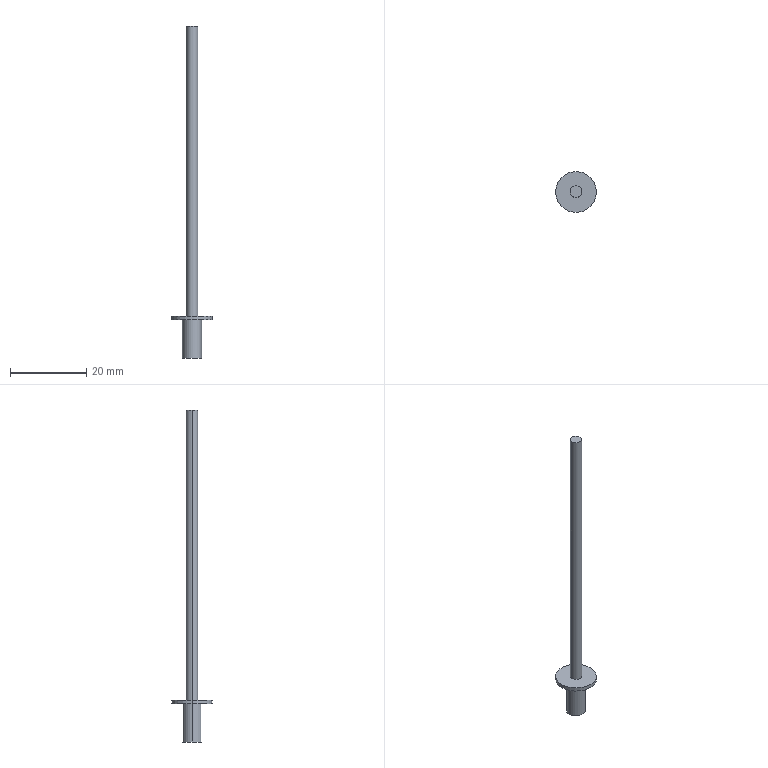Part | Creo | 1 solid | 10 faces | box 10.7 x 10.7 x 87 mm | volume 823.482 mm3 | cylinder 6 | plane 4 | commonest cylinder face diameters 3 x2 5 x2 10.7 x2
STEP:
#1=CARTESIAN_POINT('',(0.,0.,0.));
#2=DIRECTION('',(0.,0.,1.));
#3=DIRECTION('',(1.,0.,0.));
#4=AXIS2_PLACEMENT_3D('',#1,#2,#3);
#5=CARTESIAN_POINT('',(-34.3,80.134,-54.09));
#6=VERTEX_POINT('',#5);
#7=CARTESIAN_POINT('',(-31.3,80.134,-54.09));
#8=VERTEX_POINT('',#7);
#9=CARTESIAN_POINT('',(-32.8,80.134,-54.09));
#10=DIRECTION('',(0.,0.,-1.));
#11=DIRECTION('',(-1.,0.,0.));
#12=AXIS2_PLACEMENT_3D('',#9,#10,#11);
#13=CIRCLE('',#12,1.5);
#14=EDGE_CURVE('',#6,#8,#13,.T.);
#15=ORIENTED_EDGE('',*,*,#14,.T.);
#16=CARTESIAN_POINT('',(-31.3,80.134,21.91));
#17=VERTEX_POINT('',#16);
#18=CARTESIAN_POINT('',(-31.3,80.134,21.91));
#19=DIRECTION('',(0.,0.,-1.));
#20=VECTOR('',#19,76.);
#21=LINE('',#18,#20);
#22=EDGE_CURVE('',#17,#8,#21,.T.);
#23=ORIENTED_EDGE('',*,*,#22,.F.);
#24=CARTESIAN_POINT('',(-34.3,80.134,21.91));
#25=VERTEX_POINT('',#24);
#26=CARTESIAN_POINT('',(-32.8,80.134,21.91));
#27=DIRECTION('',(0.,0.,1.));
#28=DIRECTION('',(1.,0.,0.));
#29=AXIS2_PLACEMENT_3D('',#26,#27,#28);
#30=CIRCLE('',#29,1.5);
#31=EDGE_CURVE('',#17,#25,#30,.T.);
#32=ORIENTED_EDGE('',*,*,#31,.T.);
#33=CARTESIAN_POINT('',(-34.3,80.134,21.91));
#34=DIRECTION('',(0.,0.,-1.));
#35=VECTOR('',#34,76.);
#36=LINE('',#33,#35);
#37=EDGE_CURVE('',#25,#6,#36,.T.);
#38=ORIENTED_EDGE('',*,*,#37,.T.);
#39=EDGE_LOOP('',(#15,#23,#32,#38));
#40=FACE_OUTER_BOUND('',#39,.F.);
#41=CARTESIAN_POINT('',(-32.8,80.134,10.91));
#42=DIRECTION('',(0.,0.,-1.));
#43=DIRECTION('',(-1.,0.,0.));
#44=AXIS2_PLACEMENT_3D('',#41,#42,#43);
#45=CYLINDRICAL_SURFACE('',#44,1.5);
#46=ADVANCED_FACE('',(#40),#45,.T.);
#47=CARTESIAN_POINT('',(-38.15,80.134,-54.09));
#48=VERTEX_POINT('',#47);
#49=CARTESIAN_POINT('',(-27.45,80.134,-54.09));
#50=VERTEX_POINT('',#49);
#51=CARTESIAN_POINT('',(-32.8,80.134,-54.09));
#52=DIRECTION('',(0.,0.,1.));
#53=DIRECTION('',(-1.,0.,0.));
#54=AXIS2_PLACEMENT_3D('',#51,#52,#53);
#55=CIRCLE('',#54,5.35);
#56=EDGE_CURVE('',#48,#50,#55,.T.);
#57=ORIENTED_EDGE('',*,*,#56,.F.);
#58=CARTESIAN_POINT('',(-32.8,80.134,-54.09));
#59=DIRECTION('',(0.,0.,1.));
#60=DIRECTION('',(1.,0.,0.));
#61=AXIS2_PLACEMENT_3D('',#58,#59,#60);
#62=CIRCLE('',#61,5.35);
#63=EDGE_CURVE('',#50,#48,#62,.T.);
#64=ORIENTED_EDGE('',*,*,#63,.F.);
#65=EDGE_LOOP('',(#57,#64));
#66=FACE_OUTER_BOUND('',#65,.F.);
#67=ORIENTED_EDGE('',*,*,#14,.F.);
#68=CARTESIAN_POINT('',(-32.8,80.134,-54.09));
#69=DIRECTION('',(0.,0.,-1.));
#70=DIRECTION('',(1.,0.,0.));
#71=AXIS2_PLACEMENT_3D('',#68,#69,#70);
#72=CIRCLE('',#71,1.5);
#73=EDGE_CURVE('',#8,#6,#72,.T.);
#74=ORIENTED_EDGE('',*,*,#73,.F.);
#75=EDGE_LOOP('',(#67,#74));
#76=FACE_BOUND('',#75,.F.);
#77=CARTESIAN_POINT('',(0.,0.,-54.09));
#78=DIRECTION('',(0.,0.,-1.));
#79=DIRECTION('',(-1.,0.,0.));
#80=AXIS2_PLACEMENT_3D('',#77,#78,#79);
#81=PLANE('',#80);
#82=ADVANCED_FACE('',(#66,#76),#81,.F.);
#83=ORIENTED_EDGE('',*,*,#56,.T.);
#84=CARTESIAN_POINT('',(-27.45,80.134,-55.09));
#85=VERTEX_POINT('',#84);
#86=CARTESIAN_POINT('',(-27.45,80.134,-55.09));
#87=DIRECTION('',(0.,0.,1.));
#88=VECTOR('',#87,1.);
#89=LINE('',#86,#88);
#90=EDGE_CURVE('',#85,#50,#89,.T.);
#91=ORIENTED_EDGE('',*,*,#90,.F.);
#92=CARTESIAN_POINT('',(-38.15,80.134,-55.09));
#93=VERTEX_POINT('',#92);
#94=CARTESIAN_POINT('',(-32.8,80.134,-55.09));
#95=DIRECTION('',(0.,0.,-1.));
#96=DIRECTION('',(1.,0.,0.));
#97=AXIS2_PLACEMENT_3D('',#94,#95,#96);
#98=CIRCLE('',#97,5.35);
#99=EDGE_CURVE('',#85,#93,#98,.T.);
#100=ORIENTED_EDGE('',*,*,#99,.T.);
#101=CARTESIAN_POINT('',(-38.15,80.134,-55.09));
#102=DIRECTION('',(0.,0.,1.));
#103=VECTOR('',#102,1.);
#104=LINE('',#101,#103);
#105=EDGE_CURVE('',#93,#48,#104,.T.);
#106=ORIENTED_EDGE('',*,*,#105,.T.);
#107=EDGE_LOOP('',(#83,#91,#100,#106));
#108=FACE_OUTER_BOUND('',#107,.F.);
#109=CARTESIAN_POINT('',(-32.8,80.134,-104.09));
#110=DIRECTION('',(0.,0.,1.));
#111=DIRECTION('',(1.,0.,0.));
#112=AXIS2_PLACEMENT_3D('',#109,#110,#111);
#113=CYLINDRICAL_SURFACE('',#112,5.35);
#114=ADVANCED_FACE('',(#108),#113,.T.);
#115=ORIENTED_EDGE('',*,*,#63,.T.);
#116=ORIENTED_EDGE('',*,*,#105,.F.);
#117=CARTESIAN_POINT('',(-32.8,80.134,-55.09));
#118=DIRECTION('',(0.,0.,-1.));
#119=DIRECTION('',(-1.,0.,0.));
#120=AXIS2_PLACEMENT_3D('',#117,#118,#119);
#121=CIRCLE('',#120,5.35);
#122=EDGE_CURVE('',#93,#85,#121,.T.);
#123=ORIENTED_EDGE('',*,*,#122,.T.);
#124=ORIENTED_EDGE('',*,*,#90,.T.);
#125=EDGE_LOOP('',(#115,#116,#123,#124));
#126=FACE_OUTER_BOUND('',#125,.F.);
#127=CARTESIAN_POINT('',(-32.8,80.134,-104.09));
#128=DIRECTION('',(0.,0.,1.));
#129=DIRECTION('',(1.,0.,0.));
#130=AXIS2_PLACEMENT_3D('',#127,#128,#129);
#131=CYLINDRICAL_SURFACE('',#130,5.35);
#132=ADVANCED_FACE('',(#126),#131,.T.);
#133=ORIENTED_EDGE('',*,*,#122,.F.);
#134=ORIENTED_EDGE('',*,*,#99,.F.);
#135=EDGE_LOOP('',(#133,#134));
#136=FACE_OUTER_BOUND('',#135,.F.);
#137=CARTESIAN_POINT('',(-35.3,80.134,-55.09));
#138=VERTEX_POINT('',#137);
#139=CARTESIAN_POINT('',(-30.3,80.134,-55.09));
#140=VERTEX_POINT('',#139);
#141=CARTESIAN_POINT('',(-32.8,80.134,-55.09));
#142=DIRECTION('',(0.,0.,1.));
#143=DIRECTION('',(-1.,0.,0.));
#144=AXIS2_PLACEMENT_3D('',#141,#142,#143);
#145=CIRCLE('',#144,2.5);
#146=EDGE_CURVE('',#138,#140,#145,.T.);
#147=ORIENTED_EDGE('',*,*,#146,.F.);
#148=CARTESIAN_POINT('',(-32.8,80.134,-55.09));
#149=DIRECTION('',(0.,0.,1.));
#150=DIRECTION('',(1.,0.,0.));
#151=AXIS2_PLACEMENT_3D('',#148,#149,#150);
#152=CIRCLE('',#151,2.5);
#153=EDGE_CURVE('',#140,#138,#152,.T.);
#154=ORIENTED_EDGE('',*,*,#153,.F.);
#155=EDGE_LOOP('',(#147,#154));
#156=FACE_BOUND('',#155,.F.);
#157=CARTESIAN_POINT('',(0.,0.,-55.09));
#158=DIRECTION('',(0.,0.,-1.));
#159=DIRECTION('',(-1.,0.,0.));
#160=AXIS2_PLACEMENT_3D('',#157,#158,#159);
#161=PLANE('',#160);
#162=ADVANCED_FACE('',(#136,#156),#161,.T.);
#163=CARTESIAN_POINT('',(-30.3,80.134,-65.09));
#164=VERTEX_POINT('',#163);
#165=CARTESIAN_POINT('',(-35.3,80.134,-65.09));
#166=VERTEX_POINT('',#165);
#167=CARTESIAN_POINT('',(-32.8,80.134,-65.09));
#168=DIRECTION('',(0.,0.,-1.));
#169=DIRECTION('',(1.,0.,0.));
#170=AXIS2_PLACEMENT_3D('',#167,#168,#169);
#171=CIRCLE('',#170,2.5);
#172=EDGE_CURVE('',#164,#166,#171,.T.);
#173=ORIENTED_EDGE('',*,*,#172,.T.);
#174=CARTESIAN_POINT('',(-35.3,80.134,-55.09));
#175=DIRECTION('',(0.,0.,-1.));
#176=VECTOR('',#175,10.);
#177=LINE('',#174,#176);
#178=EDGE_CURVE('',#138,#166,#177,.T.);
#179=ORIENTED_EDGE('',*,*,#178,.F.);
#180=ORIENTED_EDGE('',*,*,#146,.T.);
#181=CARTESIAN_POINT('',(-30.3,80.134,-55.09));
#182=DIRECTION('',(0.,0.,-1.));
#183=VECTOR('',#182,10.);
#184=LINE('',#181,#183);
#185=EDGE_CURVE('',#140,#164,#184,.T.);
#186=ORIENTED_EDGE('',*,*,#185,.T.);
#187=EDGE_LOOP('',(#173,#179,#180,#186));
#188=FACE_OUTER_BOUND('',#187,.F.);
#189=CARTESIAN_POINT('',(-32.8,80.134,-55.09));
#190=DIRECTION('',(0.,0.,-1.));
#191=DIRECTION('',(-1.,0.,0.));
#192=AXIS2_PLACEMENT_3D('',#189,#190,#191);
#193=CYLINDRICAL_SURFACE('',#192,2.5);
#194=ADVANCED_FACE('',(#188),#193,.T.);
#195=ORIENTED_EDGE('',*,*,#172,.F.);
#196=CARTESIAN_POINT('',(-32.8,80.134,-65.09));
#197=DIRECTION('',(0.,0.,-1.));
#198=DIRECTION('',(-1.,0.,0.));
#199=AXIS2_PLACEMENT_3D('',#196,#197,#198);
#200=CIRCLE('',#199,2.5);
#201=EDGE_CURVE('',#166,#164,#200,.T.);
#202=ORIENTED_EDGE('',*,*,#201,.F.);
#203=EDGE_LOOP('',(#195,#202));
#204=FACE_OUTER_BOUND('',#203,.F.);
#205=CARTESIAN_POINT('',(-32.8,80.134,-65.09));
#206=DIRECTION('',(0.,0.,1.));
#207=DIRECTION('',(1.,0.,0.));
#208=AXIS2_PLACEMENT_3D('',#205,#206,#207);
#209=PLANE('',#208);
#210=ADVANCED_FACE('',(#204),#209,.F.);
#211=ORIENTED_EDGE('',*,*,#201,.T.);
#212=ORIENTED_EDGE('',*,*,#185,.F.);
#213=ORIENTED_EDGE('',*,*,#153,.T.);
#214=ORIENTED_EDGE('',*,*,#178,.T.);
#215=EDGE_LOOP('',(#211,#212,#213,#214));
#216=FACE_OUTER_BOUND('',#215,.F.);
#217=CARTESIAN_POINT('',(-32.8,80.134,-55.09));
#218=DIRECTION('',(0.,0.,-1.));
#219=DIRECTION('',(-1.,0.,0.));
#220=AXIS2_PLACEMENT_3D('',#217,#218,#219);
#221=CYLINDRICAL_SURFACE('',#220,2.5);
#222=ADVANCED_FACE('',(#216),#221,.T.);
#223=ORIENTED_EDGE('',*,*,#73,.T.);
#224=ORIENTED_EDGE('',*,*,#37,.F.);
#225=CARTESIAN_POINT('',(-32.8,80.134,21.91));
#226=DIRECTION('',(0.,0.,1.));
#227=DIRECTION('',(-1.,0.,0.));
#228=AXIS2_PLACEMENT_3D('',#225,#226,#227);
#229=CIRCLE('',#228,1.5);
#230=EDGE_CURVE('',#25,#17,#229,.T.);
#231=ORIENTED_EDGE('',*,*,#230,.T.);
#232=ORIENTED_EDGE('',*,*,#22,.T.);
#233=EDGE_LOOP('',(#223,#224,#231,#232));
#234=FACE_OUTER_BOUND('',#233,.F.);
#235=CARTESIAN_POINT('',(-32.8,80.134,10.91));
#236=DIRECTION('',(0.,0.,-1.));
#237=DIRECTION('',(-1.,0.,0.));
#238=AXIS2_PLACEMENT_3D('',#235,#236,#237);
#239=CYLINDRICAL_SURFACE('',#238,1.5);
#240=ADVANCED_FACE('',(#234),#239,.T.);
#241=ORIENTED_EDGE('',*,*,#31,.F.);
#242=ORIENTED_EDGE('',*,*,#230,.F.);
#243=EDGE_LOOP('',(#241,#242));
#244=FACE_OUTER_BOUND('',#243,.F.);
#245=CARTESIAN_POINT('',(33.5,-82.,21.91));
#246=DIRECTION('',(0.,0.,1.));
#247=DIRECTION('',(1.,0.,0.));
#248=AXIS2_PLACEMENT_3D('',#245,#246,#247);
#249=PLANE('',#248);
#250=ADVANCED_FACE('',(#244),#249,.T.);
#251=CLOSED_SHELL('',(#46,#82,#114,#132,#162,#194,#210,#222,#240,#250));
#252=MANIFOLD_SOLID_BREP('',#251);
#253=(LENGTH_UNIT()NAMED_UNIT(*)SI_UNIT(.MILLI.,.METRE.));
#254=UNCERTAINTY_MEASURE_WITH_UNIT(LENGTH_MEASURE(0.00883),#253,'','');
#255=(NAMED_UNIT(*)PLANE_ANGLE_UNIT()SI_UNIT($,.RADIAN.));
#256=PLANE_ANGLE_MEASURE_WITH_UNIT(PLANE_ANGLE_MEASURE(0.01745),#255);
#257=(CONVERSION_BASED_UNIT('DEGREE',#256)NAMED_UNIT(*)PLANE_ANGLE_UNIT());
#258=(NAMED_UNIT(*)SI_UNIT($,.STERADIAN.)SOLID_ANGLE_UNIT());
#259=(GEOMETRIC_REPRESENTATION_CONTEXT(3)GLOBAL_UNCERTAINTY_ASSIGNED_CONTEXT((#254))GLOBAL_UNIT_ASSIGNED_CONTEXT((#253,#257,#258))REPRESENTATION_CONTEXT('',''));
#260=ADVANCED_BREP_SHAPE_REPRESENTATION('',(#4,#252),#259);